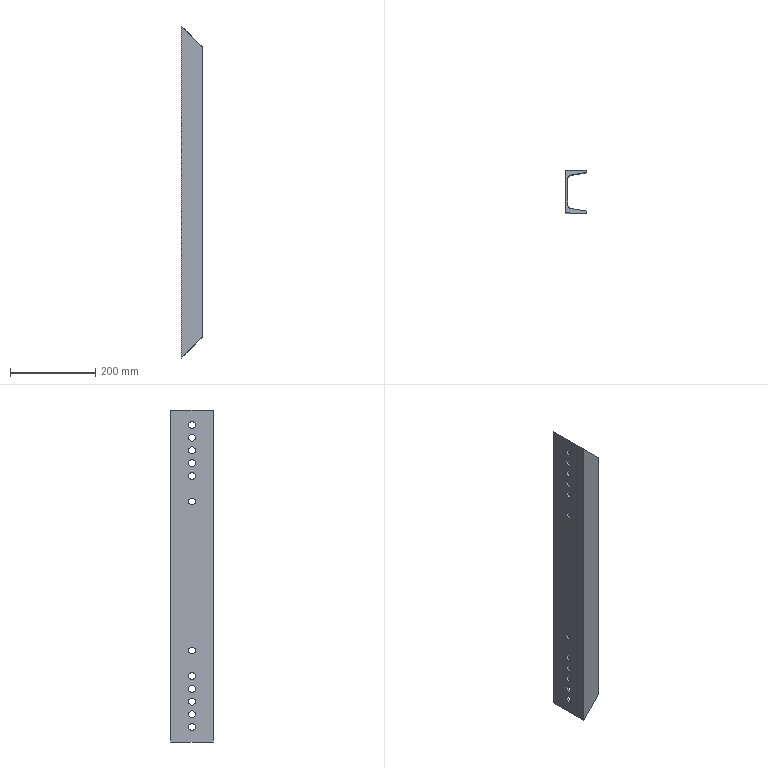Part | SolidWorks | features ICE 2, Extrusion 1 | 1 solid | 38 faces | box 50 x 100 x 780 mm | volume 980427 mm3 | cylinder 28 | plane 10 | commonest cylinder face diameters 16.5 x24 9 x2 17 x2
STEP:
#1=CARTESIAN_POINT('',(6.,-41.75,146.192));
#2=VERTEX_POINT('',#1);
#3=CARTESIAN_POINT('',(6.,-58.25,146.192));
#4=VERTEX_POINT('',#3);
#5=CARTESIAN_POINT('',(6.,-50.,146.192));
#6=DIRECTION('',(-1.,0.,0.));
#7=DIRECTION('',(0.,-1.,0.));
#8=AXIS2_PLACEMENT_3D('',#5,#6,#7);
#9=CIRCLE('',#8,8.25);
#10=EDGE_CURVE('',#2,#4,#9,.T.);
#11=ORIENTED_EDGE('',*,*,#10,.F.);
#12=CARTESIAN_POINT('',(0.,-41.75,146.192));
#13=VERTEX_POINT('',#12);
#14=CARTESIAN_POINT('',(100.,-41.75,146.192));
#15=DIRECTION('',(-1.,0.,0.));
#16=VECTOR('',#15,1000.);
#17=LINE('',#14,#16);
#18=EDGE_CURVE('',#2,#13,#17,.T.);
#19=ORIENTED_EDGE('',*,*,#18,.T.);
#20=CARTESIAN_POINT('',(0.,-58.25,146.192));
#21=VERTEX_POINT('',#20);
#22=CARTESIAN_POINT('',(0.,-50.,146.192));
#23=DIRECTION('',(-1.,0.,0.));
#24=DIRECTION('',(0.,-1.,0.));
#25=AXIS2_PLACEMENT_3D('',#22,#23,#24);
#26=CIRCLE('',#25,8.25);
#27=EDGE_CURVE('',#13,#21,#26,.T.);
#28=ORIENTED_EDGE('',*,*,#27,.T.);
#29=CARTESIAN_POINT('',(100.,-58.25,146.192));
#30=DIRECTION('',(-1.,0.,0.));
#31=VECTOR('',#30,1000.);
#32=LINE('',#29,#31);
#33=EDGE_CURVE('',#4,#21,#32,.T.);
#34=ORIENTED_EDGE('',*,*,#33,.F.);
#35=EDGE_LOOP('',(#11,#19,#28,#34));
#36=FACE_OUTER_BOUND('',#35,.T.);
#37=CARTESIAN_POINT('',(100.,-50.,146.192));
#38=DIRECTION('',(-1.,0.,0.));
#39=DIRECTION('',(0.,-1.,0.));
#40=AXIS2_PLACEMENT_3D('',#37,#38,#39);
#41=CYLINDRICAL_SURFACE('',#40,8.25);
#42=ADVANCED_FACE('',(#36),#41,.F.);
#43=CARTESIAN_POINT('',(6.,-41.75,176.192));
#44=VERTEX_POINT('',#43);
#45=CARTESIAN_POINT('',(6.,-58.25,176.192));
#46=VERTEX_POINT('',#45);
#47=CARTESIAN_POINT('',(6.,-50.,176.192));
#48=DIRECTION('',(-1.,0.,0.));
#49=DIRECTION('',(0.,-1.,0.));
#50=AXIS2_PLACEMENT_3D('',#47,#48,#49);
#51=CIRCLE('',#50,8.25);
#52=EDGE_CURVE('',#44,#46,#51,.T.);
#53=ORIENTED_EDGE('',*,*,#52,.F.);
#54=CARTESIAN_POINT('',(0.,-41.75,176.192));
#55=VERTEX_POINT('',#54);
#56=CARTESIAN_POINT('',(100.,-41.75,176.192));
#57=DIRECTION('',(-1.,0.,0.));
#58=VECTOR('',#57,1000.);
#59=LINE('',#56,#58);
#60=EDGE_CURVE('',#44,#55,#59,.T.);
#61=ORIENTED_EDGE('',*,*,#60,.T.);
#62=CARTESIAN_POINT('',(0.,-58.25,176.192));
#63=VERTEX_POINT('',#62);
#64=CARTESIAN_POINT('',(0.,-50.,176.192));
#65=DIRECTION('',(-1.,0.,0.));
#66=DIRECTION('',(0.,-1.,0.));
#67=AXIS2_PLACEMENT_3D('',#64,#65,#66);
#68=CIRCLE('',#67,8.25);
#69=EDGE_CURVE('',#55,#63,#68,.T.);
#70=ORIENTED_EDGE('',*,*,#69,.T.);
#71=CARTESIAN_POINT('',(100.,-58.25,176.192));
#72=DIRECTION('',(-1.,0.,0.));
#73=VECTOR('',#72,1000.);
#74=LINE('',#71,#73);
#75=EDGE_CURVE('',#46,#63,#74,.T.);
#76=ORIENTED_EDGE('',*,*,#75,.F.);
#77=EDGE_LOOP('',(#53,#61,#70,#76));
#78=FACE_OUTER_BOUND('',#77,.T.);
#79=CARTESIAN_POINT('',(100.,-50.,176.192));
#80=DIRECTION('',(-1.,0.,0.));
#81=DIRECTION('',(0.,-1.,0.));
#82=AXIS2_PLACEMENT_3D('',#79,#80,#81);
#83=CYLINDRICAL_SURFACE('',#82,8.25);
#84=ADVANCED_FACE('',(#78),#83,.F.);
#85=CARTESIAN_POINT('',(6.,-41.75,206.192));
#86=VERTEX_POINT('',#85);
#87=CARTESIAN_POINT('',(6.,-58.25,206.192));
#88=VERTEX_POINT('',#87);
#89=CARTESIAN_POINT('',(6.,-50.,206.192));
#90=DIRECTION('',(-1.,0.,0.));
#91=DIRECTION('',(0.,-1.,0.));
#92=AXIS2_PLACEMENT_3D('',#89,#90,#91);
#93=CIRCLE('',#92,8.25);
#94=EDGE_CURVE('',#86,#88,#93,.T.);
#95=ORIENTED_EDGE('',*,*,#94,.F.);
#96=CARTESIAN_POINT('',(0.,-41.75,206.192));
#97=VERTEX_POINT('',#96);
#98=CARTESIAN_POINT('',(100.,-41.75,206.192));
#99=DIRECTION('',(-1.,0.,0.));
#100=VECTOR('',#99,1000.);
#101=LINE('',#98,#100);
#102=EDGE_CURVE('',#86,#97,#101,.T.);
#103=ORIENTED_EDGE('',*,*,#102,.T.);
#104=CARTESIAN_POINT('',(0.,-58.25,206.192));
#105=VERTEX_POINT('',#104);
#106=CARTESIAN_POINT('',(0.,-50.,206.192));
#107=DIRECTION('',(-1.,0.,0.));
#108=DIRECTION('',(0.,-1.,0.));
#109=AXIS2_PLACEMENT_3D('',#106,#107,#108);
#110=CIRCLE('',#109,8.25);
#111=EDGE_CURVE('',#97,#105,#110,.T.);
#112=ORIENTED_EDGE('',*,*,#111,.T.);
#113=CARTESIAN_POINT('',(100.,-58.25,206.192));
#114=DIRECTION('',(-1.,0.,0.));
#115=VECTOR('',#114,1000.);
#116=LINE('',#113,#115);
#117=EDGE_CURVE('',#88,#105,#116,.T.);
#118=ORIENTED_EDGE('',*,*,#117,.F.);
#119=EDGE_LOOP('',(#95,#103,#112,#118));
#120=FACE_OUTER_BOUND('',#119,.T.);
#121=CARTESIAN_POINT('',(100.,-50.,206.192));
#122=DIRECTION('',(-1.,0.,0.));
#123=DIRECTION('',(0.,-1.,0.));
#124=AXIS2_PLACEMENT_3D('',#121,#122,#123);
#125=CYLINDRICAL_SURFACE('',#124,8.25);
#126=ADVANCED_FACE('',(#120),#125,.F.);
#127=CARTESIAN_POINT('',(6.,-41.75,236.192));
#128=VERTEX_POINT('',#127);
#129=CARTESIAN_POINT('',(6.,-58.25,236.192));
#130=VERTEX_POINT('',#129);
#131=CARTESIAN_POINT('',(6.,-50.,236.192));
#132=DIRECTION('',(-1.,0.,0.));
#133=DIRECTION('',(0.,-1.,0.));
#134=AXIS2_PLACEMENT_3D('',#131,#132,#133);
#135=CIRCLE('',#134,8.25);
#136=EDGE_CURVE('',#128,#130,#135,.T.);
#137=ORIENTED_EDGE('',*,*,#136,.F.);
#138=CARTESIAN_POINT('',(0.,-41.75,236.192));
#139=VERTEX_POINT('',#138);
#140=CARTESIAN_POINT('',(100.,-41.75,236.192));
#141=DIRECTION('',(-1.,0.,0.));
#142=VECTOR('',#141,1000.);
#143=LINE('',#140,#142);
#144=EDGE_CURVE('',#128,#139,#143,.T.);
#145=ORIENTED_EDGE('',*,*,#144,.T.);
#146=CARTESIAN_POINT('',(0.,-58.25,236.192));
#147=VERTEX_POINT('',#146);
#148=CARTESIAN_POINT('',(0.,-50.,236.192));
#149=DIRECTION('',(-1.,0.,0.));
#150=DIRECTION('',(0.,-1.,0.));
#151=AXIS2_PLACEMENT_3D('',#148,#149,#150);
#152=CIRCLE('',#151,8.25);
#153=EDGE_CURVE('',#139,#147,#152,.T.);
#154=ORIENTED_EDGE('',*,*,#153,.T.);
#155=CARTESIAN_POINT('',(100.,-58.25,236.192));
#156=DIRECTION('',(-1.,0.,0.));
#157=VECTOR('',#156,1000.);
#158=LINE('',#155,#157);
#159=EDGE_CURVE('',#130,#147,#158,.T.);
#160=ORIENTED_EDGE('',*,*,#159,.F.);
#161=EDGE_LOOP('',(#137,#145,#154,#160));
#162=FACE_OUTER_BOUND('',#161,.T.);
#163=CARTESIAN_POINT('',(100.,-50.,236.192));
#164=DIRECTION('',(-1.,0.,0.));
#165=DIRECTION('',(0.,-1.,0.));
#166=AXIS2_PLACEMENT_3D('',#163,#164,#165);
#167=CYLINDRICAL_SURFACE('',#166,8.25);
#168=ADVANCED_FACE('',(#162),#167,.F.);
#169=CARTESIAN_POINT('',(6.,-41.75,266.192));
#170=VERTEX_POINT('',#169);
#171=CARTESIAN_POINT('',(6.,-58.25,266.192));
#172=VERTEX_POINT('',#171);
#173=CARTESIAN_POINT('',(6.,-50.,266.192));
#174=DIRECTION('',(-1.,0.,0.));
#175=DIRECTION('',(0.,-1.,0.));
#176=AXIS2_PLACEMENT_3D('',#173,#174,#175);
#177=CIRCLE('',#176,8.25);
#178=EDGE_CURVE('',#170,#172,#177,.T.);
#179=ORIENTED_EDGE('',*,*,#178,.F.);
#180=CARTESIAN_POINT('',(0.,-41.75,266.192));
#181=VERTEX_POINT('',#180);
#182=CARTESIAN_POINT('',(100.,-41.75,266.192));
#183=DIRECTION('',(-1.,0.,0.));
#184=VECTOR('',#183,1000.);
#185=LINE('',#182,#184);
#186=EDGE_CURVE('',#170,#181,#185,.T.);
#187=ORIENTED_EDGE('',*,*,#186,.T.);
#188=CARTESIAN_POINT('',(0.,-58.25,266.192));
#189=VERTEX_POINT('',#188);
#190=CARTESIAN_POINT('',(0.,-50.,266.192));
#191=DIRECTION('',(-1.,0.,0.));
#192=DIRECTION('',(0.,-1.,0.));
#193=AXIS2_PLACEMENT_3D('',#190,#191,#192);
#194=CIRCLE('',#193,8.25);
#195=EDGE_CURVE('',#181,#189,#194,.T.);
#196=ORIENTED_EDGE('',*,*,#195,.T.);
#197=CARTESIAN_POINT('',(100.,-58.25,266.192));
#198=DIRECTION('',(-1.,0.,0.));
#199=VECTOR('',#198,1000.);
#200=LINE('',#197,#199);
#201=EDGE_CURVE('',#172,#189,#200,.T.);
#202=ORIENTED_EDGE('',*,*,#201,.F.);
#203=EDGE_LOOP('',(#179,#187,#196,#202));
#204=FACE_OUTER_BOUND('',#203,.T.);
#205=CARTESIAN_POINT('',(100.,-50.,266.192));
#206=DIRECTION('',(-1.,0.,0.));
#207=DIRECTION('',(0.,-1.,0.));
#208=AXIS2_PLACEMENT_3D('',#205,#206,#207);
#209=CYLINDRICAL_SURFACE('',#208,8.25);
#210=ADVANCED_FACE('',(#204),#209,.F.);
#211=CARTESIAN_POINT('',(6.,-41.75,326.192));
#212=VERTEX_POINT('',#211);
#213=CARTESIAN_POINT('',(6.,-58.25,326.192));
#214=VERTEX_POINT('',#213);
#215=CARTESIAN_POINT('',(6.,-50.,326.192));
#216=DIRECTION('',(-1.,0.,0.));
#217=DIRECTION('',(0.,-1.,0.));
#218=AXIS2_PLACEMENT_3D('',#215,#216,#217);
#219=CIRCLE('',#218,8.25);
#220=EDGE_CURVE('',#212,#214,#219,.T.);
#221=ORIENTED_EDGE('',*,*,#220,.F.);
#222=CARTESIAN_POINT('',(0.,-41.75,326.192));
#223=VERTEX_POINT('',#222);
#224=CARTESIAN_POINT('',(100.,-41.75,326.192));
#225=DIRECTION('',(-1.,0.,0.));
#226=VECTOR('',#225,1000.);
#227=LINE('',#224,#226);
#228=EDGE_CURVE('',#212,#223,#227,.T.);
#229=ORIENTED_EDGE('',*,*,#228,.T.);
#230=CARTESIAN_POINT('',(0.,-58.25,326.192));
#231=VERTEX_POINT('',#230);
#232=CARTESIAN_POINT('',(0.,-50.,326.192));
#233=DIRECTION('',(-1.,0.,0.));
#234=DIRECTION('',(0.,-1.,0.));
#235=AXIS2_PLACEMENT_3D('',#232,#233,#234);
#236=CIRCLE('',#235,8.25);
#237=EDGE_CURVE('',#223,#231,#236,.T.);
#238=ORIENTED_EDGE('',*,*,#237,.T.);
#239=CARTESIAN_POINT('',(100.,-58.25,326.192));
#240=DIRECTION('',(-1.,0.,0.));
#241=VECTOR('',#240,1000.);
#242=LINE('',#239,#241);
#243=EDGE_CURVE('',#214,#231,#242,.T.);
#244=ORIENTED_EDGE('',*,*,#243,.F.);
#245=EDGE_LOOP('',(#221,#229,#238,#244));
#246=FACE_OUTER_BOUND('',#245,.T.);
#247=CARTESIAN_POINT('',(100.,-50.,326.192));
#248=DIRECTION('',(-1.,0.,0.));
#249=DIRECTION('',(0.,-1.,0.));
#250=AXIS2_PLACEMENT_3D('',#247,#248,#249);
#251=CYLINDRICAL_SURFACE('',#250,8.25);
#252=ADVANCED_FACE('',(#246),#251,.F.);
#253=CARTESIAN_POINT('',(6.,-41.75,676.192));
#254=VERTEX_POINT('',#253);
#255=CARTESIAN_POINT('',(6.,-58.25,676.192));
#256=VERTEX_POINT('',#255);
#257=CARTESIAN_POINT('',(6.,-50.,676.192));
#258=DIRECTION('',(-1.,0.,0.));
#259=DIRECTION('',(0.,-1.,0.));
#260=AXIS2_PLACEMENT_3D('',#257,#258,#259);
#261=CIRCLE('',#260,8.25);
#262=EDGE_CURVE('',#254,#256,#261,.T.);
#263=ORIENTED_EDGE('',*,*,#262,.F.);
#264=CARTESIAN_POINT('',(0.,-41.75,676.192));
#265=VERTEX_POINT('',#264);
#266=CARTESIAN_POINT('',(100.,-41.75,676.192));
#267=DIRECTION('',(-1.,0.,0.));
#268=VECTOR('',#267,1000.);
#269=LINE('',#266,#268);
#270=EDGE_CURVE('',#254,#265,#269,.T.);
#271=ORIENTED_EDGE('',*,*,#270,.T.);
#272=CARTESIAN_POINT('',(0.,-58.25,676.192));
#273=VERTEX_POINT('',#272);
#274=CARTESIAN_POINT('',(0.,-50.,676.192));
#275=DIRECTION('',(-1.,0.,0.));
#276=DIRECTION('',(0.,1.,0.));
#277=AXIS2_PLACEMENT_3D('',#274,#275,#276);
#278=CIRCLE('',#277,8.25);
#279=EDGE_CURVE('',#265,#273,#278,.T.);
#280=ORIENTED_EDGE('',*,*,#279,.T.);
#281=CARTESIAN_POINT('',(100.,-58.25,676.192));
#282=DIRECTION('',(-1.,0.,0.));
#283=VECTOR('',#282,1000.);
#284=LINE('',#281,#283);
#285=EDGE_CURVE('',#256,#273,#284,.T.);
#286=ORIENTED_EDGE('',*,*,#285,.F.);
#287=EDGE_LOOP('',(#263,#271,#280,#286));
#288=FACE_OUTER_BOUND('',#287,.T.);
#289=CARTESIAN_POINT('',(100.,-50.,676.192));
#290=DIRECTION('',(-1.,0.,0.));
#291=DIRECTION('',(0.,-1.,0.));
#292=AXIS2_PLACEMENT_3D('',#289,#290,#291);
#293=CYLINDRICAL_SURFACE('',#292,8.25);
#294=ADVANCED_FACE('',(#288),#293,.F.);
#295=CARTESIAN_POINT('',(6.,-41.75,736.192));
#296=VERTEX_POINT('',#295);
#297=CARTESIAN_POINT('',(6.,-58.25,736.192));
#298=VERTEX_POINT('',#297);
#299=CARTESIAN_POINT('',(6.,-50.,736.192));
#300=DIRECTION('',(-1.,0.,0.));
#301=DIRECTION('',(0.,-1.,0.));
#302=AXIS2_PLACEMENT_3D('',#299,#300,#301);
#303=CIRCLE('',#302,8.25);
#304=EDGE_CURVE('',#296,#298,#303,.T.);
#305=ORIENTED_EDGE('',*,*,#304,.F.);
#306=CARTESIAN_POINT('',(0.,-41.75,736.192));
#307=VERTEX_POINT('',#306);
#308=CARTESIAN_POINT('',(100.,-41.75,736.192));
#309=DIRECTION('',(-1.,0.,0.));
#310=VECTOR('',#309,1000.);
#311=LINE('',#308,#310);
#312=EDGE_CURVE('',#296,#307,#311,.T.);
#313=ORIENTED_EDGE('',*,*,#312,.T.);
#314=CARTESIAN_POINT('',(0.,-58.25,736.192));
#315=VERTEX_POINT('',#314);
#316=CARTESIAN_POINT('',(0.,-50.,736.192));
#317=DIRECTION('',(-1.,0.,0.));
#318=DIRECTION('',(0.,1.,0.));
#319=AXIS2_PLACEMENT_3D('',#316,#317,#318);
#320=CIRCLE('',#319,8.25);
#321=EDGE_CURVE('',#307,#315,#320,.T.);
#322=ORIENTED_EDGE('',*,*,#321,.T.);
#323=CARTESIAN_POINT('',(100.,-58.25,736.192));
#324=DIRECTION('',(-1.,0.,0.));
#325=VECTOR('',#324,1000.);
#326=LINE('',#323,#325);
#327=EDGE_CURVE('',#298,#315,#326,.T.);
#328=ORIENTED_EDGE('',*,*,#327,.F.);
#329=EDGE_LOOP('',(#305,#313,#322,#328));
#330=FACE_OUTER_BOUND('',#329,.T.);
#331=CARTESIAN_POINT('',(100.,-50.,736.192));
#332=DIRECTION('',(-1.,0.,0.));
#333=DIRECTION('',(0.,-1.,0.));
#334=AXIS2_PLACEMENT_3D('',#331,#332,#333);
#335=CYLINDRICAL_SURFACE('',#334,8.25);
#336=ADVANCED_FACE('',(#330),#335,.F.);
#337=CARTESIAN_POINT('',(6.,-41.75,766.192));
#338=VERTEX_POINT('',#337);
#339=CARTESIAN_POINT('',(6.,-58.25,766.192));
#340=VERTEX_POINT('',#339);
#341=CARTESIAN_POINT('',(6.,-50.,766.192));
#342=DIRECTION('',(-1.,0.,0.));
#343=DIRECTION('',(0.,-1.,0.));
#344=AXIS2_PLACEMENT_3D('',#341,#342,#343);
#345=CIRCLE('',#344,8.25);
#346=EDGE_CURVE('',#338,#340,#345,.T.);
#347=ORIENTED_EDGE('',*,*,#346,.F.);
#348=CARTESIAN_POINT('',(0.,-41.75,766.192));
#349=VERTEX_POINT('',#348);
#350=CARTESIAN_POINT('',(100.,-41.75,766.192));
#351=DIRECTION('',(-1.,0.,0.));
#352=VECTOR('',#351,1000.);
#353=LINE('',#350,#352);
#354=EDGE_CURVE('',#338,#349,#353,.T.);
#355=ORIENTED_EDGE('',*,*,#354,.T.);
#356=CARTESIAN_POINT('',(0.,-58.25,766.192));
#357=VERTEX_POINT('',#356);
#358=CARTESIAN_POINT('',(0.,-50.,766.192));
#359=DIRECTION('',(-1.,0.,0.));
#360=DIRECTION('',(0.,1.,0.));
#361=AXIS2_PLACEMENT_3D('',#358,#359,#360);
#362=CIRCLE('',#361,8.25);
#363=EDGE_CURVE('',#349,#357,#362,.T.);
#364=ORIENTED_EDGE('',*,*,#363,.T.);
#365=CARTESIAN_POINT('',(100.,-58.25,766.192));
#366=DIRECTION('',(-1.,0.,0.));
#367=VECTOR('',#366,1000.);
#368=LINE('',#365,#367);
#369=EDGE_CURVE('',#340,#357,#368,.T.);
#370=ORIENTED_EDGE('',*,*,#369,.F.);
#371=EDGE_LOOP('',(#347,#355,#364,#370));
#372=FACE_OUTER_BOUND('',#371,.T.);
#373=CARTESIAN_POINT('',(100.,-50.,766.192));
#374=DIRECTION('',(-1.,0.,0.));
#375=DIRECTION('',(0.,-1.,0.));
#376=AXIS2_PLACEMENT_3D('',#373,#374,#375);
#377=CYLINDRICAL_SURFACE('',#376,8.25);
#378=ADVANCED_FACE('',(#372),#377,.F.);
#379=CARTESIAN_POINT('',(6.,-41.75,796.192));
#380=VERTEX_POINT('',#379);
#381=CARTESIAN_POINT('',(6.,-58.25,796.192));
#382=VERTEX_POINT('',#381);
#383=CARTESIAN_POINT('',(6.,-50.,796.192));
#384=DIRECTION('',(-1.,0.,0.));
#385=DIRECTION('',(0.,-1.,0.));
#386=AXIS2_PLACEMENT_3D('',#383,#384,#385);
#387=CIRCLE('',#386,8.25);
#388=EDGE_CURVE('',#380,#382,#387,.T.);
#389=ORIENTED_EDGE('',*,*,#388,.F.);
#390=CARTESIAN_POINT('',(0.,-41.75,796.192));
#391=VERTEX_POINT('',#390);
#392=CARTESIAN_POINT('',(100.,-41.75,796.192));
#393=DIRECTION('',(-1.,0.,0.));
#394=VECTOR('',#393,1000.);
#395=LINE('',#392,#394);
#396=EDGE_CURVE('',#380,#391,#395,.T.);
#397=ORIENTED_EDGE('',*,*,#396,.T.);
#398=CARTESIAN_POINT('',(0.,-58.25,796.192));
#399=VERTEX_POINT('',#398);
#400=CARTESIAN_POINT('',(0.,-50.,796.192));
#401=DIRECTION('',(-1.,0.,0.));
#402=DIRECTION('',(0.,1.,0.));
#403=AXIS2_PLACEMENT_3D('',#400,#401,#402);
#404=CIRCLE('',#403,8.25);
#405=EDGE_CURVE('',#391,#399,#404,.T.);
#406=ORIENTED_EDGE('',*,*,#405,.T.);
#407=CARTESIAN_POINT('',(100.,-58.25,796.192));
#408=DIRECTION('',(-1.,0.,0.));
#409=VECTOR('',#408,1000.);
#410=LINE('',#407,#409);
#411=EDGE_CURVE('',#382,#399,#410,.T.);
#412=ORIENTED_EDGE('',*,*,#411,.F.);
#413=EDGE_LOOP('',(#389,#397,#406,#412));
#414=FACE_OUTER_BOUND('',#413,.T.);
#415=CARTESIAN_POINT('',(100.,-50.,796.192));
#416=DIRECTION('',(-1.,0.,0.));
#417=DIRECTION('',(0.,-1.,0.));
#418=AXIS2_PLACEMENT_3D('',#415,#416,#417);
#419=CYLINDRICAL_SURFACE('',#418,8.25);
#420=ADVANCED_FACE('',(#414),#419,.F.);
#421=CARTESIAN_POINT('',(6.,-41.75,826.192));
#422=VERTEX_POINT('',#421);
#423=CARTESIAN_POINT('',(6.,-58.25,826.192));
#424=VERTEX_POINT('',#423);
#425=CARTESIAN_POINT('',(6.,-50.,826.192));
#426=DIRECTION('',(-1.,0.,0.));
#427=DIRECTION('',(0.,-1.,0.));
#428=AXIS2_PLACEMENT_3D('',#425,#426,#427);
#429=CIRCLE('',#428,8.25);
#430=EDGE_CURVE('',#422,#424,#429,.T.);
#431=ORIENTED_EDGE('',*,*,#430,.F.);
#432=CARTESIAN_POINT('',(0.,-41.75,826.192));
#433=VERTEX_POINT('',#432);
#434=CARTESIAN_POINT('',(100.,-41.75,826.192));
#435=DIRECTION('',(-1.,0.,0.));
#436=VECTOR('',#435,1000.);
#437=LINE('',#434,#436);
#438=EDGE_CURVE('',#422,#433,#437,.T.);
#439=ORIENTED_EDGE('',*,*,#438,.T.);
#440=CARTESIAN_POINT('',(0.,-58.25,826.192));
#441=VERTEX_POINT('',#440);
#442=CARTESIAN_POINT('',(0.,-50.,826.192));
#443=DIRECTION('',(-1.,0.,0.));
#444=DIRECTION('',(0.,1.,0.));
#445=AXIS2_PLACEMENT_3D('',#442,#443,#444);
#446=CIRCLE('',#445,8.25);
#447=EDGE_CURVE('',#433,#441,#446,.T.);
#448=ORIENTED_EDGE('',*,*,#447,.T.);
#449=CARTESIAN_POINT('',(100.,-58.25,826.192));
#450=DIRECTION('',(-1.,0.,0.));
#451=VECTOR('',#450,1000.);
#452=LINE('',#449,#451);
#453=EDGE_CURVE('',#424,#441,#452,.T.);
#454=ORIENTED_EDGE('',*,*,#453,.F.);
#455=EDGE_LOOP('',(#431,#439,#448,#454));
#456=FACE_OUTER_BOUND('',#455,.T.);
#457=CARTESIAN_POINT('',(100.,-50.,826.192));
#458=DIRECTION('',(-1.,0.,0.));
#459=DIRECTION('',(0.,-1.,0.));
#460=AXIS2_PLACEMENT_3D('',#457,#458,#459);
#461=CYLINDRICAL_SURFACE('',#460,8.25);
#462=ADVANCED_FACE('',(#456),#461,.F.);
#463=CARTESIAN_POINT('',(6.,-41.75,856.192));
#464=VERTEX_POINT('',#463);
#465=CARTESIAN_POINT('',(6.,-58.25,856.192));
#466=VERTEX_POINT('',#465);
#467=CARTESIAN_POINT('',(6.,-50.,856.192));
#468=DIRECTION('',(-1.,0.,0.));
#469=DIRECTION('',(0.,-1.,0.));
#470=AXIS2_PLACEMENT_3D('',#467,#468,#469);
#471=CIRCLE('',#470,8.25);
#472=EDGE_CURVE('',#464,#466,#471,.T.);
#473=ORIENTED_EDGE('',*,*,#472,.F.);
#474=CARTESIAN_POINT('',(0.,-41.75,856.192));
#475=VERTEX_POINT('',#474);
#476=CARTESIAN_POINT('',(100.,-41.75,856.192));
#477=DIRECTION('',(-1.,0.,0.));
#478=VECTOR('',#477,1000.);
#479=LINE('',#476,#478);
#480=EDGE_CURVE('',#464,#475,#479,.T.);
#481=ORIENTED_EDGE('',*,*,#480,.T.);
#482=CARTESIAN_POINT('',(0.,-58.25,856.192));
#483=VERTEX_POINT('',#482);
#484=CARTESIAN_POINT('',(0.,-50.,856.192));
#485=DIRECTION('',(-1.,0.,0.));
#486=DIRECTION('',(0.,1.,0.));
#487=AXIS2_PLACEMENT_3D('',#484,#485,#486);
#488=CIRCLE('',#487,8.25);
#489=EDGE_CURVE('',#475,#483,#488,.T.);
#490=ORIENTED_EDGE('',*,*,#489,.T.);
#491=CARTESIAN_POINT('',(100.,-58.25,856.192));
#492=DIRECTION('',(-1.,0.,0.));
#493=VECTOR('',#492,1000.);
#494=LINE('',#491,#493);
#495=EDGE_CURVE('',#466,#483,#494,.T.);
#496=ORIENTED_EDGE('',*,*,#495,.F.);
#497=EDGE_LOOP('',(#473,#481,#490,#496));
#498=FACE_OUTER_BOUND('',#497,.T.);
#499=CARTESIAN_POINT('',(100.,-50.,856.192));
#500=DIRECTION('',(-1.,0.,0.));
#501=DIRECTION('',(0.,-1.,0.));
#502=AXIS2_PLACEMENT_3D('',#499,#500,#501);
#503=CYLINDRICAL_SURFACE('',#502,8.25);
#504=ADVANCED_FACE('',(#498),#503,.F.);
#505=CARTESIAN_POINT('',(50.,0.,841.192));
#506=VERTEX_POINT('',#505);
#507=CARTESIAN_POINT('',(50.,0.,161.192));
#508=VERTEX_POINT('',#507);
#509=CARTESIAN_POINT('',(50.,0.,1000.));
#510=DIRECTION('',(0.,0.,-1.));
#511=VECTOR('',#510,1000.);
#512=LINE('',#509,#511);
#513=EDGE_CURVE('',#506,#508,#512,.T.);
#514=ORIENTED_EDGE('',*,*,#513,.T.);
#515=CARTESIAN_POINT('',(0.,0.,111.192));
#516=VERTEX_POINT('',#515);
#517=CARTESIAN_POINT('',(0.,0.,111.192));
#518=DIRECTION('',(0.7071,0.,0.7071));
#519=VECTOR('',#518,1000.);
#520=LINE('',#517,#519);
#521=EDGE_CURVE('',#516,#508,#520,.T.);
#522=ORIENTED_EDGE('',*,*,#521,.F.);
#523=CARTESIAN_POINT('',(0.,0.,891.192));
#524=VERTEX_POINT('',#523);
#525=CARTESIAN_POINT('',(0.,0.,1000.));
#526=DIRECTION('',(0.,0.,-1.));
#527=VECTOR('',#526,1000.);
#528=LINE('',#525,#527);
#529=EDGE_CURVE('',#524,#516,#528,.T.);
#530=ORIENTED_EDGE('',*,*,#529,.F.);
#531=CARTESIAN_POINT('',(197.399,0.,693.793));
#532=DIRECTION('',(-0.7071,0.,0.7071));
#533=VECTOR('',#532,1000.);
#534=LINE('',#531,#533);
#535=EDGE_CURVE('',#506,#524,#534,.T.);
#536=ORIENTED_EDGE('',*,*,#535,.F.);
#537=EDGE_LOOP('',(#514,#522,#530,#536));
#538=FACE_OUTER_BOUND('',#537,.T.);
#539=CARTESIAN_POINT('',(0.,0.,1000.));
#540=DIRECTION('',(0.,-1.,0.));
#541=DIRECTION('',(0.,0.,-1.));
#542=AXIS2_PLACEMENT_3D('',#539,#540,#541);
#543=PLANE('',#542);
#544=ADVANCED_FACE('',(#538),#543,.F.);
#545=CARTESIAN_POINT('',(0.,-50.,146.192));
#546=DIRECTION('',(-1.,0.,0.));
#547=DIRECTION('',(0.,-1.,0.));
#548=AXIS2_PLACEMENT_3D('',#545,#546,#547);
#549=CIRCLE('',#548,8.25);
#550=EDGE_CURVE('',#21,#13,#549,.T.);
#551=ORIENTED_EDGE('',*,*,#550,.F.);
#552=ORIENTED_EDGE('',*,*,#27,.F.);
#553=EDGE_LOOP('',(#551,#552));
#554=FACE_BOUND('',#553,.T.);
#555=CARTESIAN_POINT('',(0.,-50.,176.192));
#556=DIRECTION('',(-1.,0.,0.));
#557=DIRECTION('',(0.,-1.,0.));
#558=AXIS2_PLACEMENT_3D('',#555,#556,#557);
#559=CIRCLE('',#558,8.25);
#560=EDGE_CURVE('',#63,#55,#559,.T.);
#561=ORIENTED_EDGE('',*,*,#560,.F.);
#562=ORIENTED_EDGE('',*,*,#69,.F.);
#563=EDGE_LOOP('',(#561,#562));
#564=FACE_BOUND('',#563,.T.);
#565=CARTESIAN_POINT('',(0.,-50.,206.192));
#566=DIRECTION('',(-1.,0.,0.));
#567=DIRECTION('',(0.,-1.,0.));
#568=AXIS2_PLACEMENT_3D('',#565,#566,#567);
#569=CIRCLE('',#568,8.25);
#570=EDGE_CURVE('',#105,#97,#569,.T.);
#571=ORIENTED_EDGE('',*,*,#570,.F.);
#572=ORIENTED_EDGE('',*,*,#111,.F.);
#573=EDGE_LOOP('',(#571,#572));
#574=FACE_BOUND('',#573,.T.);
#575=CARTESIAN_POINT('',(0.,-50.,236.192));
#576=DIRECTION('',(-1.,0.,0.));
#577=DIRECTION('',(0.,-1.,0.));
#578=AXIS2_PLACEMENT_3D('',#575,#576,#577);
#579=CIRCLE('',#578,8.25);
#580=EDGE_CURVE('',#147,#139,#579,.T.);
#581=ORIENTED_EDGE('',*,*,#580,.F.);
#582=ORIENTED_EDGE('',*,*,#153,.F.);
#583=EDGE_LOOP('',(#581,#582));
#584=FACE_BOUND('',#583,.T.);
#585=CARTESIAN_POINT('',(0.,-50.,266.192));
#586=DIRECTION('',(-1.,0.,0.));
#587=DIRECTION('',(0.,-1.,0.));
#588=AXIS2_PLACEMENT_3D('',#585,#586,#587);
#589=CIRCLE('',#588,8.25);
#590=EDGE_CURVE('',#189,#181,#589,.T.);
#591=ORIENTED_EDGE('',*,*,#590,.F.);
#592=ORIENTED_EDGE('',*,*,#195,.F.);
#593=EDGE_LOOP('',(#591,#592));
#594=FACE_BOUND('',#593,.T.);
#595=CARTESIAN_POINT('',(0.,-50.,326.192));
#596=DIRECTION('',(-1.,0.,0.));
#597=DIRECTION('',(0.,-1.,0.));
#598=AXIS2_PLACEMENT_3D('',#595,#596,#597);
#599=CIRCLE('',#598,8.25);
#600=EDGE_CURVE('',#231,#223,#599,.T.);
#601=ORIENTED_EDGE('',*,*,#600,.F.);
#602=ORIENTED_EDGE('',*,*,#237,.F.);
#603=EDGE_LOOP('',(#601,#602));
#604=FACE_BOUND('',#603,.T.);
#605=CARTESIAN_POINT('',(0.,-50.,676.192));
#606=DIRECTION('',(-1.,0.,0.));
#607=DIRECTION('',(0.,1.,0.));
#608=AXIS2_PLACEMENT_3D('',#605,#606,#607);
#609=CIRCLE('',#608,8.25);
#610=EDGE_CURVE('',#273,#265,#609,.T.);
#611=ORIENTED_EDGE('',*,*,#610,.F.);
#612=ORIENTED_EDGE('',*,*,#279,.F.);
#613=EDGE_LOOP('',(#611,#612));
#614=FACE_BOUND('',#613,.T.);
#615=CARTESIAN_POINT('',(0.,-50.,736.192));
#616=DIRECTION('',(-1.,0.,0.));
#617=DIRECTION('',(0.,1.,0.));
#618=AXIS2_PLACEMENT_3D('',#615,#616,#617);
#619=CIRCLE('',#618,8.25);
#620=EDGE_CURVE('',#315,#307,#619,.T.);
#621=ORIENTED_EDGE('',*,*,#620,.F.);
#622=ORIENTED_EDGE('',*,*,#321,.F.);
#623=EDGE_LOOP('',(#621,#622));
#624=FACE_BOUND('',#623,.T.);
#625=CARTESIAN_POINT('',(0.,-50.,766.192));
#626=DIRECTION('',(-1.,0.,0.));
#627=DIRECTION('',(0.,1.,0.));
#628=AXIS2_PLACEMENT_3D('',#625,#626,#627);
#629=CIRCLE('',#628,8.25);
#630=EDGE_CURVE('',#357,#349,#629,.T.);
#631=ORIENTED_EDGE('',*,*,#630,.F.);
#632=ORIENTED_EDGE('',*,*,#363,.F.);
#633=EDGE_LOOP('',(#631,#632));
#634=FACE_BOUND('',#633,.T.);
#635=CARTESIAN_POINT('',(0.,-50.,796.192));
#636=DIRECTION('',(-1.,0.,0.));
#637=DIRECTION('',(0.,1.,0.));
#638=AXIS2_PLACEMENT_3D('',#635,#636,#637);
#639=CIRCLE('',#638,8.25);
#640=EDGE_CURVE('',#399,#391,#639,.T.);
#641=ORIENTED_EDGE('',*,*,#640,.F.);
#642=ORIENTED_EDGE('',*,*,#405,.F.);
#643=EDGE_LOOP('',(#641,#642));
#644=FACE_BOUND('',#643,.T.);
#645=CARTESIAN_POINT('',(0.,-50.,826.192));
#646=DIRECTION('',(-1.,0.,0.));
#647=DIRECTION('',(0.,1.,0.));
#648=AXIS2_PLACEMENT_3D('',#645,#646,#647);
#649=CIRCLE('',#648,8.25);
#650=EDGE_CURVE('',#441,#433,#649,.T.);
#651=ORIENTED_EDGE('',*,*,#650,.F.);
#652=ORIENTED_EDGE('',*,*,#447,.F.);
#653=EDGE_LOOP('',(#651,#652));
#654=FACE_BOUND('',#653,.T.);
#655=CARTESIAN_POINT('',(0.,-50.,856.192));
#656=DIRECTION('',(-1.,0.,0.));
#657=DIRECTION('',(0.,1.,0.));
#658=AXIS2_PLACEMENT_3D('',#655,#656,#657);
#659=CIRCLE('',#658,8.25);
#660=EDGE_CURVE('',#483,#475,#659,.T.);
#661=ORIENTED_EDGE('',*,*,#660,.F.);
#662=ORIENTED_EDGE('',*,*,#489,.F.);
#663=EDGE_LOOP('',(#661,#662));
#664=FACE_BOUND('',#663,.T.);
#665=ORIENTED_EDGE('',*,*,#529,.T.);
#666=CARTESIAN_POINT('',(0.,-100.,111.192));
#667=VERTEX_POINT('',#666);
#668=CARTESIAN_POINT('',(0.,-100.,111.192));
#669=DIRECTION('',(0.,1.,0.));
#670=VECTOR('',#669,1000.);
#671=LINE('',#668,#670);
#672=EDGE_CURVE('',#667,#516,#671,.T.);
#673=ORIENTED_EDGE('',*,*,#672,.F.);
#674=CARTESIAN_POINT('',(0.,-100.,891.192));
#675=VERTEX_POINT('',#674);
#676=CARTESIAN_POINT('',(0.,-100.,1000.));
#677=DIRECTION('',(0.,0.,-1.));
#678=VECTOR('',#677,1000.);
#679=LINE('',#676,#678);
#680=EDGE_CURVE('',#675,#667,#679,.T.);
#681=ORIENTED_EDGE('',*,*,#680,.F.);
#682=CARTESIAN_POINT('',(0.,-100.,891.192));
#683=DIRECTION('',(0.,1.,0.));
#684=VECTOR('',#683,1000.);
#685=LINE('',#682,#684);
#686=EDGE_CURVE('',#675,#524,#685,.T.);
#687=ORIENTED_EDGE('',*,*,#686,.T.);
#688=EDGE_LOOP('',(#665,#673,#681,#687));
#689=FACE_OUTER_BOUND('',#688,.T.);
#690=CARTESIAN_POINT('',(0.,0.,1000.));
#691=DIRECTION('',(1.,0.,0.));
#692=DIRECTION('',(0.,1.,0.));
#693=AXIS2_PLACEMENT_3D('',#690,#691,#692);
#694=PLANE('',#693);
#695=ADVANCED_FACE('',(#554,#564,#574,#584,#594,#604,#614,#624,#634,#644,#654,#664,#689),#694,.F.);
#696=ORIENTED_EDGE('',*,*,#680,.T.);
#697=CARTESIAN_POINT('',(50.,-100.,161.192));
#698=VERTEX_POINT('',#697);
#699=CARTESIAN_POINT('',(0.,-100.,111.192));
#700=DIRECTION('',(0.7071,0.,0.7071));
#701=VECTOR('',#700,1000.);
#702=LINE('',#699,#701);
#703=EDGE_CURVE('',#667,#698,#702,.T.);
#704=ORIENTED_EDGE('',*,*,#703,.T.);
#705=CARTESIAN_POINT('',(50.,-100.,841.192));
#706=VERTEX_POINT('',#705);
#707=CARTESIAN_POINT('',(50.,-100.,1000.));
#708=DIRECTION('',(0.,0.,-1.));
#709=VECTOR('',#708,1000.);
#710=LINE('',#707,#709);
#711=EDGE_CURVE('',#706,#698,#710,.T.);
#712=ORIENTED_EDGE('',*,*,#711,.F.);
#713=CARTESIAN_POINT('',(197.399,-100.,693.793));
#714=DIRECTION('',(-0.7071,0.,0.7071));
#715=VECTOR('',#714,1000.);
#716=LINE('',#713,#715);
#717=EDGE_CURVE('',#706,#675,#716,.T.);
#718=ORIENTED_EDGE('',*,*,#717,.T.);
#719=EDGE_LOOP('',(#696,#704,#712,#718));
#720=FACE_OUTER_BOUND('',#719,.T.);
#721=CARTESIAN_POINT('',(0.,-100.,1000.));
#722=DIRECTION('',(0.,1.,0.));
#723=DIRECTION('',(0.,0.,1.));
#724=AXIS2_PLACEMENT_3D('',#721,#722,#723);
#725=PLANE('',#724);
#726=ADVANCED_FACE('',(#720),#725,.F.);
#727=ORIENTED_EDGE('',*,*,#711,.T.);
#728=CARTESIAN_POINT('',(50.,-98.925,161.192));
#729=VERTEX_POINT('',#728);
#730=CARTESIAN_POINT('',(50.,-100.,161.192));
#731=DIRECTION('',(0.,1.,0.));
#732=VECTOR('',#731,1000.);
#733=LINE('',#730,#732);
#734=EDGE_CURVE('',#698,#729,#733,.T.);
#735=ORIENTED_EDGE('',*,*,#734,.T.);
#736=CARTESIAN_POINT('',(50.,-98.925,841.192));
#737=VERTEX_POINT('',#736);
#738=CARTESIAN_POINT('',(50.,-98.925,1000.));
#739=DIRECTION('',(0.,0.,-1.));
#740=VECTOR('',#739,1000.);
#741=LINE('',#738,#740);
#742=EDGE_CURVE('',#737,#729,#741,.T.);
#743=ORIENTED_EDGE('',*,*,#742,.F.);
#744=CARTESIAN_POINT('',(50.,-100.,841.192));
#745=DIRECTION('',(0.,-1.,0.));
#746=VECTOR('',#745,1000.);
#747=LINE('',#744,#746);
#748=EDGE_CURVE('',#737,#706,#747,.T.);
#749=ORIENTED_EDGE('',*,*,#748,.T.);
#750=EDGE_LOOP('',(#727,#735,#743,#749));
#751=FACE_OUTER_BOUND('',#750,.T.);
#752=CARTESIAN_POINT('',(50.,-100.,1000.));
#753=DIRECTION('',(-1.,0.,0.));
#754=DIRECTION('',(0.,0.,1.));
#755=AXIS2_PLACEMENT_3D('',#752,#753,#754);
#756=PLANE('',#755);
#757=ADVANCED_FACE('',(#751),#756,.F.);
#758=ORIENTED_EDGE('',*,*,#742,.T.);
#759=CARTESIAN_POINT('',(46.126,-94.469,157.319));
#760=VERTEX_POINT('',#759);
#761=CARTESIAN_POINT('',(50.,-98.925,161.192));
#762=CARTESIAN_POINT('',(50.,-96.572,161.192));
#763=CARTESIAN_POINT('',(48.456,-94.797,159.649));
#764=CARTESIAN_POINT('',(46.126,-94.469,157.319));
#765=(BOUNDED_CURVE()B_SPLINE_CURVE(3,(#761,#762,#763,#764),.UNSPECIFIED.,.F.,.F.)B_SPLINE_CURVE_WITH_KNOTS((4,4),(3.142,4.573),.UNSPECIFIED.)CURVE()GEOMETRIC_REPRESENTATION_ITEM()RATIONAL_B_SPLINE_CURVE((1.,0.8365,0.8365,1.))REPRESENTATION_ITEM(''));
#766=EDGE_CURVE('',#729,#760,#765,.T.);
#767=ORIENTED_EDGE('',*,*,#766,.T.);
#768=CARTESIAN_POINT('',(46.126,-94.469,845.066));
#769=VERTEX_POINT('',#768);
#770=CARTESIAN_POINT('',(46.126,-94.469,1000.));
#771=DIRECTION('',(0.,0.,-1.));
#772=VECTOR('',#771,1000.);
#773=LINE('',#770,#772);
#774=EDGE_CURVE('',#769,#760,#773,.T.);
#775=ORIENTED_EDGE('',*,*,#774,.F.);
#776=CARTESIAN_POINT('',(46.126,-94.469,845.066));
#777=CARTESIAN_POINT('',(48.456,-94.797,842.736));
#778=CARTESIAN_POINT('',(50.,-96.572,841.192));
#779=CARTESIAN_POINT('',(50.,-98.925,841.192));
#780=(BOUNDED_CURVE()B_SPLINE_CURVE(3,(#776,#777,#778,#779),.UNSPECIFIED.,.F.,.T.)B_SPLINE_CURVE_WITH_KNOTS((4,4),(4.852,6.283),.UNSPECIFIED.)CURVE()GEOMETRIC_REPRESENTATION_ITEM()RATIONAL_B_SPLINE_CURVE((1.,0.8365,0.8365,1.))REPRESENTATION_ITEM(''));
#781=EDGE_CURVE('',#769,#737,#780,.T.);
#782=ORIENTED_EDGE('',*,*,#781,.T.);
#783=EDGE_LOOP('',(#758,#767,#775,#782));
#784=FACE_OUTER_BOUND('',#783,.T.);
#785=CARTESIAN_POINT('',(45.5,-98.925,1000.));
#786=DIRECTION('',(0.,0.,-1.));
#787=DIRECTION('',(-1.,0.,0.));
#788=AXIS2_PLACEMENT_3D('',#785,#786,#787);
#789=CYLINDRICAL_SURFACE('',#788,4.5);
#790=ADVANCED_FACE('',(#784),#789,.T.);
#791=ORIENTED_EDGE('',*,*,#774,.T.);
#792=CARTESIAN_POINT('',(13.317,-89.858,124.509));
#793=VERTEX_POINT('',#792);
#794=CARTESIAN_POINT('',(446.782,-150.778,557.974));
#795=DIRECTION('',(-0.7036,0.09889,-0.7036));
#796=VECTOR('',#795,1000.);
#797=LINE('',#794,#796);
#798=EDGE_CURVE('',#760,#793,#797,.T.);
#799=ORIENTED_EDGE('',*,*,#798,.T.);
#800=CARTESIAN_POINT('',(13.317,-89.858,877.875));
#801=VERTEX_POINT('',#800);
#802=CARTESIAN_POINT('',(13.317,-89.858,1000.));
#803=DIRECTION('',(0.,0.,-1.));
#804=VECTOR('',#803,1000.);
#805=LINE('',#802,#804);
#806=EDGE_CURVE('',#801,#793,#805,.T.);
#807=ORIENTED_EDGE('',*,*,#806,.F.);
#808=CARTESIAN_POINT('',(-47.148,-81.36,938.34));
#809=DIRECTION('',(0.7036,-0.09889,-0.7036));
#810=VECTOR('',#809,1000.);
#811=LINE('',#808,#810);
#812=EDGE_CURVE('',#801,#769,#811,.T.);
#813=ORIENTED_EDGE('',*,*,#812,.T.);
#814=EDGE_LOOP('',(#791,#799,#807,#813));
#815=FACE_OUTER_BOUND('',#814,.T.);
#816=CARTESIAN_POINT('',(13.317,-89.858,1000.));
#817=DIRECTION('',(-0.1392,-0.9903,0.));
#818=DIRECTION('',(0.9903,-0.1392,0.));
#819=AXIS2_PLACEMENT_3D('',#816,#817,#818);
#820=PLANE('',#819);
#821=ADVANCED_FACE('',(#815),#820,.F.);
#822=ORIENTED_EDGE('',*,*,#806,.T.);
#823=CARTESIAN_POINT('',(6.,-81.441,117.192));
#824=VERTEX_POINT('',#823);
#825=CARTESIAN_POINT('',(13.317,-89.858,124.509));
#826=CARTESIAN_POINT('',(8.916,-89.24,120.108));
#827=CARTESIAN_POINT('',(6.,-85.885,117.192));
#828=CARTESIAN_POINT('',(6.,-81.441,117.192));
#829=(BOUNDED_CURVE()B_SPLINE_CURVE(3,(#825,#826,#827,#828),.UNSPECIFIED.,.F.,.F.)B_SPLINE_CURVE_WITH_KNOTS((4,4),(4.852,6.283),.UNSPECIFIED.)CURVE()GEOMETRIC_REPRESENTATION_ITEM()RATIONAL_B_SPLINE_CURVE((1.,0.8365,0.8365,1.))REPRESENTATION_ITEM(''));
#830=EDGE_CURVE('',#793,#824,#829,.T.);
#831=ORIENTED_EDGE('',*,*,#830,.T.);
#832=CARTESIAN_POINT('',(6.,-81.441,885.192));
#833=VERTEX_POINT('',#832);
#834=CARTESIAN_POINT('',(6.,-81.441,1000.));
#835=DIRECTION('',(0.,0.,-1.));
#836=VECTOR('',#835,1000.);
#837=LINE('',#834,#836);
#838=EDGE_CURVE('',#833,#824,#837,.T.);
#839=ORIENTED_EDGE('',*,*,#838,.F.);
#840=CARTESIAN_POINT('',(6.,-81.441,885.192));
#841=CARTESIAN_POINT('',(6.,-85.885,885.192));
#842=CARTESIAN_POINT('',(8.916,-89.24,882.276));
#843=CARTESIAN_POINT('',(13.317,-89.858,877.875));
#844=(BOUNDED_CURVE()B_SPLINE_CURVE(3,(#840,#841,#842,#843),.UNSPECIFIED.,.F.,.F.)B_SPLINE_CURVE_WITH_KNOTS((4,4),(3.142,4.573),.UNSPECIFIED.)CURVE()GEOMETRIC_REPRESENTATION_ITEM()RATIONAL_B_SPLINE_CURVE((1.,0.8365,0.8365,1.))REPRESENTATION_ITEM(''));
#845=EDGE_CURVE('',#833,#801,#844,.T.);
#846=ORIENTED_EDGE('',*,*,#845,.T.);
#847=EDGE_LOOP('',(#822,#831,#839,#846));
#848=FACE_OUTER_BOUND('',#847,.T.);
#849=CARTESIAN_POINT('',(14.5,-81.441,1000.));
#850=DIRECTION('',(0.,0.,-1.));
#851=DIRECTION('',(-1.,0.,0.));
#852=AXIS2_PLACEMENT_3D('',#849,#850,#851);
#853=CYLINDRICAL_SURFACE('',#852,8.5);
#854=ADVANCED_FACE('',(#848),#853,.F.);
#855=CARTESIAN_POINT('',(6.,-50.,146.192));
#856=DIRECTION('',(-1.,0.,0.));
#857=DIRECTION('',(0.,-1.,0.));
#858=AXIS2_PLACEMENT_3D('',#855,#856,#857);
#859=CIRCLE('',#858,8.25);
#860=EDGE_CURVE('',#4,#2,#859,.T.);
#861=ORIENTED_EDGE('',*,*,#860,.T.);
#862=ORIENTED_EDGE('',*,*,#10,.T.);
#863=EDGE_LOOP('',(#861,#862));
#864=FACE_BOUND('',#863,.T.);
#865=CARTESIAN_POINT('',(6.,-50.,176.192));
#866=DIRECTION('',(-1.,0.,0.));
#867=DIRECTION('',(0.,-1.,0.));
#868=AXIS2_PLACEMENT_3D('',#865,#866,#867);
#869=CIRCLE('',#868,8.25);
#870=EDGE_CURVE('',#46,#44,#869,.T.);
#871=ORIENTED_EDGE('',*,*,#870,.T.);
#872=ORIENTED_EDGE('',*,*,#52,.T.);
#873=EDGE_LOOP('',(#871,#872));
#874=FACE_BOUND('',#873,.T.);
#875=CARTESIAN_POINT('',(6.,-50.,206.192));
#876=DIRECTION('',(-1.,0.,0.));
#877=DIRECTION('',(0.,-1.,0.));
#878=AXIS2_PLACEMENT_3D('',#875,#876,#877);
#879=CIRCLE('',#878,8.25);
#880=EDGE_CURVE('',#88,#86,#879,.T.);
#881=ORIENTED_EDGE('',*,*,#880,.T.);
#882=ORIENTED_EDGE('',*,*,#94,.T.);
#883=EDGE_LOOP('',(#881,#882));
#884=FACE_BOUND('',#883,.T.);
#885=CARTESIAN_POINT('',(6.,-50.,236.192));
#886=DIRECTION('',(-1.,0.,0.));
#887=DIRECTION('',(0.,-1.,0.));
#888=AXIS2_PLACEMENT_3D('',#885,#886,#887);
#889=CIRCLE('',#888,8.25);
#890=EDGE_CURVE('',#130,#128,#889,.T.);
#891=ORIENTED_EDGE('',*,*,#890,.T.);
#892=ORIENTED_EDGE('',*,*,#136,.T.);
#893=EDGE_LOOP('',(#891,#892));
#894=FACE_BOUND('',#893,.T.);
#895=CARTESIAN_POINT('',(6.,-50.,266.192));
#896=DIRECTION('',(-1.,0.,0.));
#897=DIRECTION('',(0.,-1.,0.));
#898=AXIS2_PLACEMENT_3D('',#895,#896,#897);
#899=CIRCLE('',#898,8.25);
#900=EDGE_CURVE('',#172,#170,#899,.T.);
#901=ORIENTED_EDGE('',*,*,#900,.T.);
#902=ORIENTED_EDGE('',*,*,#178,.T.);
#903=EDGE_LOOP('',(#901,#902));
#904=FACE_BOUND('',#903,.T.);
#905=CARTESIAN_POINT('',(6.,-50.,326.192));
#906=DIRECTION('',(-1.,0.,0.));
#907=DIRECTION('',(0.,-1.,0.));
#908=AXIS2_PLACEMENT_3D('',#905,#906,#907);
#909=CIRCLE('',#908,8.25);
#910=EDGE_CURVE('',#214,#212,#909,.T.);
#911=ORIENTED_EDGE('',*,*,#910,.T.);
#912=ORIENTED_EDGE('',*,*,#220,.T.);
#913=EDGE_LOOP('',(#911,#912));
#914=FACE_BOUND('',#913,.T.);
#915=CARTESIAN_POINT('',(6.,-50.,676.192));
#916=DIRECTION('',(-1.,0.,0.));
#917=DIRECTION('',(0.,-1.,0.));
#918=AXIS2_PLACEMENT_3D('',#915,#916,#917);
#919=CIRCLE('',#918,8.25);
#920=EDGE_CURVE('',#256,#254,#919,.T.);
#921=ORIENTED_EDGE('',*,*,#920,.T.);
#922=ORIENTED_EDGE('',*,*,#262,.T.);
#923=EDGE_LOOP('',(#921,#922));
#924=FACE_BOUND('',#923,.T.);
#925=CARTESIAN_POINT('',(6.,-50.,736.192));
#926=DIRECTION('',(-1.,0.,0.));
#927=DIRECTION('',(0.,-1.,0.));
#928=AXIS2_PLACEMENT_3D('',#925,#926,#927);
#929=CIRCLE('',#928,8.25);
#930=EDGE_CURVE('',#298,#296,#929,.T.);
#931=ORIENTED_EDGE('',*,*,#930,.T.);
#932=ORIENTED_EDGE('',*,*,#304,.T.);
#933=EDGE_LOOP('',(#931,#932));
#934=FACE_BOUND('',#933,.T.);
#935=CARTESIAN_POINT('',(6.,-50.,766.192));
#936=DIRECTION('',(-1.,0.,0.));
#937=DIRECTION('',(0.,-1.,0.));
#938=AXIS2_PLACEMENT_3D('',#935,#936,#937);
#939=CIRCLE('',#938,8.25);
#940=EDGE_CURVE('',#340,#338,#939,.T.);
#941=ORIENTED_EDGE('',*,*,#940,.T.);
#942=ORIENTED_EDGE('',*,*,#346,.T.);
#943=EDGE_LOOP('',(#941,#942));
#944=FACE_BOUND('',#943,.T.);
#945=CARTESIAN_POINT('',(6.,-50.,796.192));
#946=DIRECTION('',(-1.,0.,0.));
#947=DIRECTION('',(0.,-1.,0.));
#948=AXIS2_PLACEMENT_3D('',#945,#946,#947);
#949=CIRCLE('',#948,8.25);
#950=EDGE_CURVE('',#382,#380,#949,.T.);
#951=ORIENTED_EDGE('',*,*,#950,.T.);
#952=ORIENTED_EDGE('',*,*,#388,.T.);
#953=EDGE_LOOP('',(#951,#952));
#954=FACE_BOUND('',#953,.T.);
#955=CARTESIAN_POINT('',(6.,-50.,826.192));
#956=DIRECTION('',(-1.,0.,0.));
#957=DIRECTION('',(0.,-1.,0.));
#958=AXIS2_PLACEMENT_3D('',#955,#956,#957);
#959=CIRCLE('',#958,8.25);
#960=EDGE_CURVE('',#424,#422,#959,.T.);
#961=ORIENTED_EDGE('',*,*,#960,.T.);
#962=ORIENTED_EDGE('',*,*,#430,.T.);
#963=EDGE_LOOP('',(#961,#962));
#964=FACE_BOUND('',#963,.T.);
#965=CARTESIAN_POINT('',(6.,-50.,856.192));
#966=DIRECTION('',(-1.,0.,0.));
#967=DIRECTION('',(0.,-1.,0.));
#968=AXIS2_PLACEMENT_3D('',#965,#966,#967);
#969=CIRCLE('',#968,8.25);
#970=EDGE_CURVE('',#466,#464,#969,.T.);
#971=ORIENTED_EDGE('',*,*,#970,.T.);
#972=ORIENTED_EDGE('',*,*,#472,.T.);
#973=EDGE_LOOP('',(#971,#972));
#974=FACE_BOUND('',#973,.T.);
#975=ORIENTED_EDGE('',*,*,#838,.T.);
#976=CARTESIAN_POINT('',(6.,-18.559,117.192));
#977=VERTEX_POINT('',#976);
#978=CARTESIAN_POINT('',(6.,-18.559,117.192));
#979=DIRECTION('',(0.,1.,0.));
#980=VECTOR('',#979,1000.);
#981=LINE('',#978,#980);
#982=EDGE_CURVE('',#824,#977,#981,.T.);
#983=ORIENTED_EDGE('',*,*,#982,.T.);
#984=CARTESIAN_POINT('',(6.,-18.559,885.192));
#985=VERTEX_POINT('',#984);
#986=CARTESIAN_POINT('',(6.,-18.559,1000.));
#987=DIRECTION('',(0.,0.,-1.));
#988=VECTOR('',#987,1000.);
#989=LINE('',#986,#988);
#990=EDGE_CURVE('',#985,#977,#989,.T.);
#991=ORIENTED_EDGE('',*,*,#990,.F.);
#992=CARTESIAN_POINT('',(6.,-18.559,885.192));
#993=DIRECTION('',(0.,-1.,0.));
#994=VECTOR('',#993,1000.);
#995=LINE('',#992,#994);
#996=EDGE_CURVE('',#985,#833,#995,.T.);
#997=ORIENTED_EDGE('',*,*,#996,.T.);
#998=EDGE_LOOP('',(#975,#983,#991,#997));
#999=FACE_OUTER_BOUND('',#998,.T.);
#1000=CARTESIAN_POINT('',(6.,-18.559,1000.));
#1001=DIRECTION('',(-1.,0.,0.));
#1002=DIRECTION('',(0.,-1.,0.));
#1003=AXIS2_PLACEMENT_3D('',#1000,#1001,#1002);
#1004=PLANE('',#1003);
#1005=ADVANCED_FACE('',(#864,#874,#884,#894,#904,#914,#924,#934,#944,#954,#964,#974,#999),#1004,.F.);
#1006=ORIENTED_EDGE('',*,*,#990,.T.);
#1007=CARTESIAN_POINT('',(13.317,-10.142,124.509));
#1008=VERTEX_POINT('',#1007);
#1009=CARTESIAN_POINT('',(6.,-18.559,117.192));
#1010=CARTESIAN_POINT('',(6.,-14.115,117.192));
#1011=CARTESIAN_POINT('',(8.916,-10.76,120.108));
#1012=CARTESIAN_POINT('',(13.317,-10.142,124.509));
#1013=(BOUNDED_CURVE()B_SPLINE_CURVE(3,(#1009,#1010,#1011,#1012),.UNSPECIFIED.,.F.,.F.)B_SPLINE_CURVE_WITH_KNOTS((4,4),(0.,1.431),.UNSPECIFIED.)CURVE()GEOMETRIC_REPRESENTATION_ITEM()RATIONAL_B_SPLINE_CURVE((1.,0.8365,0.8365,1.))REPRESENTATION_ITEM(''));
#1014=EDGE_CURVE('',#977,#1008,#1013,.T.);
#1015=ORIENTED_EDGE('',*,*,#1014,.T.);
#1016=CARTESIAN_POINT('',(13.317,-10.142,877.875));
#1017=VERTEX_POINT('',#1016);
#1018=CARTESIAN_POINT('',(13.317,-10.142,1000.));
#1019=DIRECTION('',(0.,0.,-1.));
#1020=VECTOR('',#1019,1000.);
#1021=LINE('',#1018,#1020);
#1022=EDGE_CURVE('',#1017,#1008,#1021,.T.);
#1023=ORIENTED_EDGE('',*,*,#1022,.F.);
#1024=CARTESIAN_POINT('',(13.317,-10.142,877.875));
#1025=CARTESIAN_POINT('',(8.916,-10.76,882.276));
#1026=CARTESIAN_POINT('',(6.,-14.115,885.192));
#1027=CARTESIAN_POINT('',(6.,-18.559,885.192));
#1028=(BOUNDED_CURVE()B_SPLINE_CURVE(3,(#1024,#1025,#1026,#1027),.UNSPECIFIED.,.F.,.F.)B_SPLINE_CURVE_WITH_KNOTS((4,4),(1.71,3.142),.UNSPECIFIED.)CURVE()GEOMETRIC_REPRESENTATION_ITEM()RATIONAL_B_SPLINE_CURVE((1.,0.8365,0.8365,1.))REPRESENTATION_ITEM(''));
#1029=EDGE_CURVE('',#1017,#985,#1028,.T.);
#1030=ORIENTED_EDGE('',*,*,#1029,.T.);
#1031=EDGE_LOOP('',(#1006,#1015,#1023,#1030));
#1032=FACE_OUTER_BOUND('',#1031,.T.);
#1033=CARTESIAN_POINT('',(14.5,-18.559,1000.));
#1034=DIRECTION('',(0.,0.,-1.));
#1035=DIRECTION('',(-1.,0.,0.));
#1036=AXIS2_PLACEMENT_3D('',#1033,#1034,#1035);
#1037=CYLINDRICAL_SURFACE('',#1036,8.5);
#1038=ADVANCED_FACE('',(#1032),#1037,.F.);
#1039=ORIENTED_EDGE('',*,*,#1022,.T.);
#1040=CARTESIAN_POINT('',(46.126,-5.531,157.319));
#1041=VERTEX_POINT('',#1040);
#1042=CARTESIAN_POINT('',(463.347,53.106,574.539));
#1043=DIRECTION('',(0.7036,0.09889,0.7036));
#1044=VECTOR('',#1043,1000.);
#1045=LINE('',#1042,#1044);
#1046=EDGE_CURVE('',#1008,#1041,#1045,.T.);
#1047=ORIENTED_EDGE('',*,*,#1046,.T.);
#1048=CARTESIAN_POINT('',(46.126,-5.531,845.066));
#1049=VERTEX_POINT('',#1048);
#1050=CARTESIAN_POINT('',(46.126,-5.531,1000.));
#1051=DIRECTION('',(0.,0.,-1.));
#1052=VECTOR('',#1051,1000.);
#1053=LINE('',#1050,#1052);
#1054=EDGE_CURVE('',#1049,#1041,#1053,.T.);
#1055=ORIENTED_EDGE('',*,*,#1054,.F.);
#1056=CARTESIAN_POINT('',(-30.583,-16.312,921.775));
#1057=DIRECTION('',(-0.7036,-0.09889,0.7036));
#1058=VECTOR('',#1057,1000.);
#1059=LINE('',#1056,#1058);
#1060=EDGE_CURVE('',#1049,#1017,#1059,.T.);
#1061=ORIENTED_EDGE('',*,*,#1060,.T.);
#1062=EDGE_LOOP('',(#1039,#1047,#1055,#1061));
#1063=FACE_OUTER_BOUND('',#1062,.T.);
#1064=CARTESIAN_POINT('',(46.126,-5.531,1000.));
#1065=DIRECTION('',(-0.1392,0.9903,0.));
#1066=DIRECTION('',(-0.9903,-0.1392,0.));
#1067=AXIS2_PLACEMENT_3D('',#1064,#1065,#1066);
#1068=PLANE('',#1067);
#1069=ADVANCED_FACE('',(#1063),#1068,.F.);
#1070=ORIENTED_EDGE('',*,*,#1054,.T.);
#1071=CARTESIAN_POINT('',(50.,-1.075,161.192));
#1072=VERTEX_POINT('',#1071);
#1073=CARTESIAN_POINT('',(46.126,-5.531,157.319));
#1074=CARTESIAN_POINT('',(48.456,-5.203,159.649));
#1075=CARTESIAN_POINT('',(50.,-3.428,161.192));
#1076=CARTESIAN_POINT('',(50.,-1.075,161.192));
#1077=(BOUNDED_CURVE()B_SPLINE_CURVE(3,(#1073,#1074,#1075,#1076),.UNSPECIFIED.,.F.,.F.)B_SPLINE_CURVE_WITH_KNOTS((4,4),(1.71,3.142),.UNSPECIFIED.)CURVE()GEOMETRIC_REPRESENTATION_ITEM()RATIONAL_B_SPLINE_CURVE((1.,0.8365,0.8365,1.))REPRESENTATION_ITEM(''));
#1078=EDGE_CURVE('',#1041,#1072,#1077,.T.);
#1079=ORIENTED_EDGE('',*,*,#1078,.T.);
#1080=CARTESIAN_POINT('',(50.,-1.075,841.192));
#1081=VERTEX_POINT('',#1080);
#1082=CARTESIAN_POINT('',(50.,-1.075,1000.));
#1083=DIRECTION('',(0.,0.,-1.));
#1084=VECTOR('',#1083,1000.);
#1085=LINE('',#1082,#1084);
#1086=EDGE_CURVE('',#1081,#1072,#1085,.T.);
#1087=ORIENTED_EDGE('',*,*,#1086,.F.);
#1088=CARTESIAN_POINT('',(50.,-1.075,841.192));
#1089=CARTESIAN_POINT('',(50.,-3.428,841.192));
#1090=CARTESIAN_POINT('',(48.456,-5.203,842.736));
#1091=CARTESIAN_POINT('',(46.126,-5.531,845.066));
#1092=(BOUNDED_CURVE()B_SPLINE_CURVE(3,(#1088,#1089,#1090,#1091),.UNSPECIFIED.,.F.,.F.)B_SPLINE_CURVE_WITH_KNOTS((4,4),(0.,1.431),.UNSPECIFIED.)CURVE()GEOMETRIC_REPRESENTATION_ITEM()RATIONAL_B_SPLINE_CURVE((1.,0.8365,0.8365,1.))REPRESENTATION_ITEM(''));
#1093=EDGE_CURVE('',#1081,#1049,#1092,.T.);
#1094=ORIENTED_EDGE('',*,*,#1093,.T.);
#1095=EDGE_LOOP('',(#1070,#1079,#1087,#1094));
#1096=FACE_OUTER_BOUND('',#1095,.T.);
#1097=CARTESIAN_POINT('',(45.5,-1.075,1000.));
#1098=DIRECTION('',(0.,0.,-1.));
#1099=DIRECTION('',(-1.,0.,0.));
#1100=AXIS2_PLACEMENT_3D('',#1097,#1098,#1099);
#1101=CYLINDRICAL_SURFACE('',#1100,4.5);
#1102=ADVANCED_FACE('',(#1096),#1101,.T.);
#1103=ORIENTED_EDGE('',*,*,#1086,.T.);
#1104=CARTESIAN_POINT('',(50.,0.,161.192));
#1105=DIRECTION('',(0.,1.,0.));
#1106=VECTOR('',#1105,1000.);
#1107=LINE('',#1104,#1106);
#1108=EDGE_CURVE('',#1072,#508,#1107,.T.);
#1109=ORIENTED_EDGE('',*,*,#1108,.T.);
#1110=ORIENTED_EDGE('',*,*,#513,.F.);
#1111=CARTESIAN_POINT('',(50.,0.,841.192));
#1112=DIRECTION('',(0.,-1.,0.));
#1113=VECTOR('',#1112,1000.);
#1114=LINE('',#1111,#1113);
#1115=EDGE_CURVE('',#506,#1081,#1114,.T.);
#1116=ORIENTED_EDGE('',*,*,#1115,.T.);
#1117=EDGE_LOOP('',(#1103,#1109,#1110,#1116));
#1118=FACE_OUTER_BOUND('',#1117,.T.);
#1119=CARTESIAN_POINT('',(50.,0.,1000.));
#1120=DIRECTION('',(-1.,0.,0.));
#1121=DIRECTION('',(0.,0.,1.));
#1122=AXIS2_PLACEMENT_3D('',#1119,#1120,#1121);
#1123=PLANE('',#1122);
#1124=ADVANCED_FACE('',(#1118),#1123,.F.);
#1125=ORIENTED_EDGE('',*,*,#781,.F.);
#1126=ORIENTED_EDGE('',*,*,#812,.F.);
#1127=ORIENTED_EDGE('',*,*,#845,.F.);
#1128=ORIENTED_EDGE('',*,*,#996,.F.);
#1129=ORIENTED_EDGE('',*,*,#1029,.F.);
#1130=ORIENTED_EDGE('',*,*,#1060,.F.);
#1131=ORIENTED_EDGE('',*,*,#1093,.F.);
#1132=ORIENTED_EDGE('',*,*,#1115,.F.);
#1133=ORIENTED_EDGE('',*,*,#535,.T.);
#1134=ORIENTED_EDGE('',*,*,#686,.F.);
#1135=ORIENTED_EDGE('',*,*,#717,.F.);
#1136=ORIENTED_EDGE('',*,*,#748,.F.);
#1137=EDGE_LOOP('',(#1125,#1126,#1127,#1128,#1129,#1130,#1131,#1132,#1133,#1134,#1135,#1136));
#1138=FACE_OUTER_BOUND('',#1137,.T.);
#1139=CARTESIAN_POINT('',(197.399,-100.,693.793));
#1140=DIRECTION('',(-0.7071,0.,-0.7071));
#1141=DIRECTION('',(-0.7071,0.,0.7071));
#1142=AXIS2_PLACEMENT_3D('',#1139,#1140,#1141);
#1143=PLANE('',#1142);
#1144=ADVANCED_FACE('',(#1138),#1143,.F.);
#1145=ORIENTED_EDGE('',*,*,#703,.F.);
#1146=ORIENTED_EDGE('',*,*,#672,.T.);
#1147=ORIENTED_EDGE('',*,*,#521,.T.);
#1148=ORIENTED_EDGE('',*,*,#1108,.F.);
#1149=ORIENTED_EDGE('',*,*,#1078,.F.);
#1150=ORIENTED_EDGE('',*,*,#1046,.F.);
#1151=ORIENTED_EDGE('',*,*,#1014,.F.);
#1152=ORIENTED_EDGE('',*,*,#982,.F.);
#1153=ORIENTED_EDGE('',*,*,#830,.F.);
#1154=ORIENTED_EDGE('',*,*,#798,.F.);
#1155=ORIENTED_EDGE('',*,*,#766,.F.);
#1156=ORIENTED_EDGE('',*,*,#734,.F.);
#1157=EDGE_LOOP('',(#1145,#1146,#1147,#1148,#1149,#1150,#1151,#1152,#1153,#1154,#1155,#1156));
#1158=FACE_OUTER_BOUND('',#1157,.T.);
#1159=CARTESIAN_POINT('',(0.,-100.,111.192));
#1160=DIRECTION('',(-0.7071,0.,0.7071));
#1161=DIRECTION('',(0.7071,0.,0.7071));
#1162=AXIS2_PLACEMENT_3D('',#1159,#1160,#1161);
#1163=PLANE('',#1162);
#1164=ADVANCED_FACE('',(#1158),#1163,.F.);
#1165=ORIENTED_EDGE('',*,*,#480,.F.);
#1166=ORIENTED_EDGE('',*,*,#970,.F.);
#1167=ORIENTED_EDGE('',*,*,#495,.T.);
#1168=ORIENTED_EDGE('',*,*,#660,.T.);
#1169=EDGE_LOOP('',(#1165,#1166,#1167,#1168));
#1170=FACE_OUTER_BOUND('',#1169,.T.);
#1171=CARTESIAN_POINT('',(100.,-50.,856.192));
#1172=DIRECTION('',(-1.,0.,0.));
#1173=DIRECTION('',(0.,-1.,0.));
#1174=AXIS2_PLACEMENT_3D('',#1171,#1172,#1173);
#1175=CYLINDRICAL_SURFACE('',#1174,8.25);
#1176=ADVANCED_FACE('',(#1170),#1175,.F.);
#1177=ORIENTED_EDGE('',*,*,#438,.F.);
#1178=ORIENTED_EDGE('',*,*,#960,.F.);
#1179=ORIENTED_EDGE('',*,*,#453,.T.);
#1180=ORIENTED_EDGE('',*,*,#650,.T.);
#1181=EDGE_LOOP('',(#1177,#1178,#1179,#1180));
#1182=FACE_OUTER_BOUND('',#1181,.T.);
#1183=CARTESIAN_POINT('',(100.,-50.,826.192));
#1184=DIRECTION('',(-1.,0.,0.));
#1185=DIRECTION('',(0.,-1.,0.));
#1186=AXIS2_PLACEMENT_3D('',#1183,#1184,#1185);
#1187=CYLINDRICAL_SURFACE('',#1186,8.25);
#1188=ADVANCED_FACE('',(#1182),#1187,.F.);
#1189=ORIENTED_EDGE('',*,*,#396,.F.);
#1190=ORIENTED_EDGE('',*,*,#950,.F.);
#1191=ORIENTED_EDGE('',*,*,#411,.T.);
#1192=ORIENTED_EDGE('',*,*,#640,.T.);
#1193=EDGE_LOOP('',(#1189,#1190,#1191,#1192));
#1194=FACE_OUTER_BOUND('',#1193,.T.);
#1195=CARTESIAN_POINT('',(100.,-50.,796.192));
#1196=DIRECTION('',(-1.,0.,0.));
#1197=DIRECTION('',(0.,-1.,0.));
#1198=AXIS2_PLACEMENT_3D('',#1195,#1196,#1197);
#1199=CYLINDRICAL_SURFACE('',#1198,8.25);
#1200=ADVANCED_FACE('',(#1194),#1199,.F.);
#1201=ORIENTED_EDGE('',*,*,#354,.F.);
#1202=ORIENTED_EDGE('',*,*,#940,.F.);
#1203=ORIENTED_EDGE('',*,*,#369,.T.);
#1204=ORIENTED_EDGE('',*,*,#630,.T.);
#1205=EDGE_LOOP('',(#1201,#1202,#1203,#1204));
#1206=FACE_OUTER_BOUND('',#1205,.T.);
#1207=CARTESIAN_POINT('',(100.,-50.,766.192));
#1208=DIRECTION('',(-1.,0.,0.));
#1209=DIRECTION('',(0.,-1.,0.));
#1210=AXIS2_PLACEMENT_3D('',#1207,#1208,#1209);
#1211=CYLINDRICAL_SURFACE('',#1210,8.25);
#1212=ADVANCED_FACE('',(#1206),#1211,.F.);
#1213=ORIENTED_EDGE('',*,*,#312,.F.);
#1214=ORIENTED_EDGE('',*,*,#930,.F.);
#1215=ORIENTED_EDGE('',*,*,#327,.T.);
#1216=ORIENTED_EDGE('',*,*,#620,.T.);
#1217=EDGE_LOOP('',(#1213,#1214,#1215,#1216));
#1218=FACE_OUTER_BOUND('',#1217,.T.);
#1219=CARTESIAN_POINT('',(100.,-50.,736.192));
#1220=DIRECTION('',(-1.,0.,0.));
#1221=DIRECTION('',(0.,-1.,0.));
#1222=AXIS2_PLACEMENT_3D('',#1219,#1220,#1221);
#1223=CYLINDRICAL_SURFACE('',#1222,8.25);
#1224=ADVANCED_FACE('',(#1218),#1223,.F.);
#1225=ORIENTED_EDGE('',*,*,#270,.F.);
#1226=ORIENTED_EDGE('',*,*,#920,.F.);
#1227=ORIENTED_EDGE('',*,*,#285,.T.);
#1228=ORIENTED_EDGE('',*,*,#610,.T.);
#1229=EDGE_LOOP('',(#1225,#1226,#1227,#1228));
#1230=FACE_OUTER_BOUND('',#1229,.T.);
#1231=CARTESIAN_POINT('',(100.,-50.,676.192));
#1232=DIRECTION('',(-1.,0.,0.));
#1233=DIRECTION('',(0.,-1.,0.));
#1234=AXIS2_PLACEMENT_3D('',#1231,#1232,#1233);
#1235=CYLINDRICAL_SURFACE('',#1234,8.25);
#1236=ADVANCED_FACE('',(#1230),#1235,.F.);
#1237=ORIENTED_EDGE('',*,*,#228,.F.);
#1238=ORIENTED_EDGE('',*,*,#910,.F.);
#1239=ORIENTED_EDGE('',*,*,#243,.T.);
#1240=ORIENTED_EDGE('',*,*,#600,.T.);
#1241=EDGE_LOOP('',(#1237,#1238,#1239,#1240));
#1242=FACE_OUTER_BOUND('',#1241,.T.);
#1243=CARTESIAN_POINT('',(100.,-50.,326.192));
#1244=DIRECTION('',(-1.,0.,0.));
#1245=DIRECTION('',(0.,-1.,0.));
#1246=AXIS2_PLACEMENT_3D('',#1243,#1244,#1245);
#1247=CYLINDRICAL_SURFACE('',#1246,8.25);
#1248=ADVANCED_FACE('',(#1242),#1247,.F.);
#1249=ORIENTED_EDGE('',*,*,#186,.F.);
#1250=ORIENTED_EDGE('',*,*,#900,.F.);
#1251=ORIENTED_EDGE('',*,*,#201,.T.);
#1252=ORIENTED_EDGE('',*,*,#590,.T.);
#1253=EDGE_LOOP('',(#1249,#1250,#1251,#1252));
#1254=FACE_OUTER_BOUND('',#1253,.T.);
#1255=CARTESIAN_POINT('',(100.,-50.,266.192));
#1256=DIRECTION('',(-1.,0.,0.));
#1257=DIRECTION('',(0.,-1.,0.));
#1258=AXIS2_PLACEMENT_3D('',#1255,#1256,#1257);
#1259=CYLINDRICAL_SURFACE('',#1258,8.25);
#1260=ADVANCED_FACE('',(#1254),#1259,.F.);
#1261=ORIENTED_EDGE('',*,*,#144,.F.);
#1262=ORIENTED_EDGE('',*,*,#890,.F.);
#1263=ORIENTED_EDGE('',*,*,#159,.T.);
#1264=ORIENTED_EDGE('',*,*,#580,.T.);
#1265=EDGE_LOOP('',(#1261,#1262,#1263,#1264));
#1266=FACE_OUTER_BOUND('',#1265,.T.);
#1267=CARTESIAN_POINT('',(100.,-50.,236.192));
#1268=DIRECTION('',(-1.,0.,0.));
#1269=DIRECTION('',(0.,-1.,0.));
#1270=AXIS2_PLACEMENT_3D('',#1267,#1268,#1269);
#1271=CYLINDRICAL_SURFACE('',#1270,8.25);
#1272=ADVANCED_FACE('',(#1266),#1271,.F.);
#1273=ORIENTED_EDGE('',*,*,#102,.F.);
#1274=ORIENTED_EDGE('',*,*,#880,.F.);
#1275=ORIENTED_EDGE('',*,*,#117,.T.);
#1276=ORIENTED_EDGE('',*,*,#570,.T.);
#1277=EDGE_LOOP('',(#1273,#1274,#1275,#1276));
#1278=FACE_OUTER_BOUND('',#1277,.T.);
#1279=CARTESIAN_POINT('',(100.,-50.,206.192));
#1280=DIRECTION('',(-1.,0.,0.));
#1281=DIRECTION('',(0.,-1.,0.));
#1282=AXIS2_PLACEMENT_3D('',#1279,#1280,#1281);
#1283=CYLINDRICAL_SURFACE('',#1282,8.25);
#1284=ADVANCED_FACE('',(#1278),#1283,.F.);
#1285=ORIENTED_EDGE('',*,*,#60,.F.);
#1286=ORIENTED_EDGE('',*,*,#870,.F.);
#1287=ORIENTED_EDGE('',*,*,#75,.T.);
#1288=ORIENTED_EDGE('',*,*,#560,.T.);
#1289=EDGE_LOOP('',(#1285,#1286,#1287,#1288));
#1290=FACE_OUTER_BOUND('',#1289,.T.);
#1291=CARTESIAN_POINT('',(100.,-50.,176.192));
#1292=DIRECTION('',(-1.,0.,0.));
#1293=DIRECTION('',(0.,-1.,0.));
#1294=AXIS2_PLACEMENT_3D('',#1291,#1292,#1293);
#1295=CYLINDRICAL_SURFACE('',#1294,8.25);
#1296=ADVANCED_FACE('',(#1290),#1295,.F.);
#1297=ORIENTED_EDGE('',*,*,#18,.F.);
#1298=ORIENTED_EDGE('',*,*,#860,.F.);
#1299=ORIENTED_EDGE('',*,*,#33,.T.);
#1300=ORIENTED_EDGE('',*,*,#550,.T.);
#1301=EDGE_LOOP('',(#1297,#1298,#1299,#1300));
#1302=FACE_OUTER_BOUND('',#1301,.T.);
#1303=CARTESIAN_POINT('',(100.,-50.,146.192));
#1304=DIRECTION('',(-1.,0.,0.));
#1305=DIRECTION('',(0.,-1.,0.));
#1306=AXIS2_PLACEMENT_3D('',#1303,#1304,#1305);
#1307=CYLINDRICAL_SURFACE('',#1306,8.25);
#1308=ADVANCED_FACE('',(#1302),#1307,.F.);
#1309=CLOSED_SHELL('',(#42,#84,#126,#168,#210,#252,#294,#336,#378,#420,#462,#504,#544,#695,#726,#757,#790,#821,#854,#1005,#1038,#1069,#1102,#1124,#1144,#1164,#1176,#1188,#1200,#1212,#1224,#1236,#1248,#1260,#1272,#1284,#1296,#1308));
#1310=MANIFOLD_SOLID_BREP('',#1309);
#1311=CARTESIAN_POINT('',(0.,0.,0.));
#1312=DIRECTION('',(0.,0.,1.));
#1313=DIRECTION('',(1.,0.,0.));
#1314=AXIS2_PLACEMENT_3D('',#1311,#1312,#1313);
#1315=(LENGTH_UNIT()NAMED_UNIT(*)SI_UNIT(.MILLI.,.METRE.));
#1316=UNCERTAINTY_MEASURE_WITH_UNIT(LENGTH_MEASURE(0.00001),#1315,'','');
#1317=(NAMED_UNIT(*)PLANE_ANGLE_UNIT()SI_UNIT($,.RADIAN.));
#1318=(NAMED_UNIT(*)SI_UNIT($,.STERADIAN.)SOLID_ANGLE_UNIT());
#1319=(GEOMETRIC_REPRESENTATION_CONTEXT(3)GLOBAL_UNCERTAINTY_ASSIGNED_CONTEXT((#1316))GLOBAL_UNIT_ASSIGNED_CONTEXT((#1315,#1317,#1318))REPRESENTATION_CONTEXT('',''));
#1320=ADVANCED_BREP_SHAPE_REPRESENTATION('',(#1310,#1314),#1319);